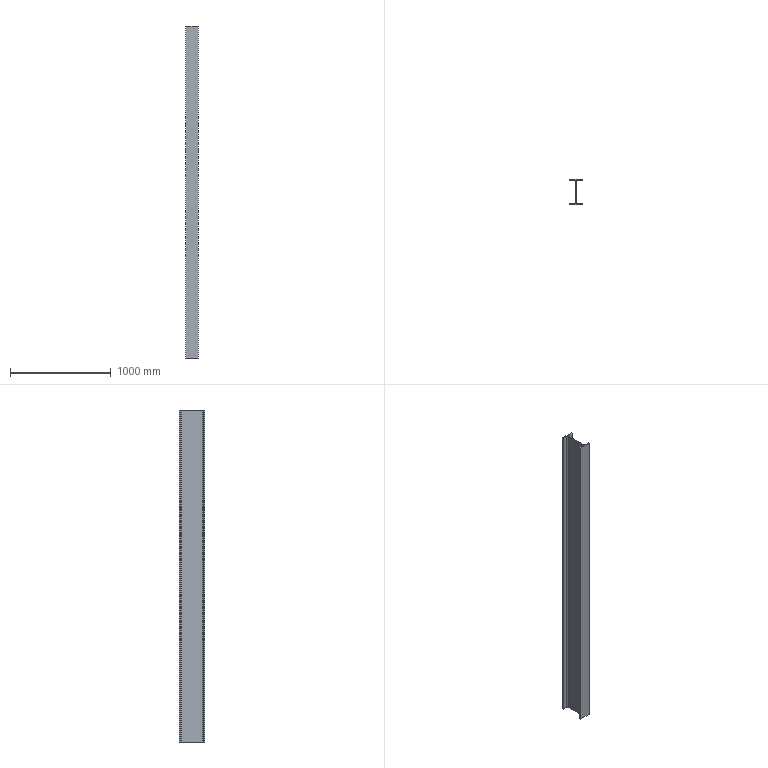Part | SolidWorks | features Extrusion 1 | 1 solid | 18 faces | box 125 x 250 x 3300 mm | volume 12199896 mm3 | plane 14 | cylinder 4 | commonest cylinder face diameters 16 x4
STEP:
#1=CARTESIAN_POINT('',(-62.5,9.,0.));
#2=VERTEX_POINT('',#1);
#3=CARTESIAN_POINT('',(-62.5,0.,0.));
#4=VERTEX_POINT('',#3);
#5=CARTESIAN_POINT('',(-62.5,0.,0.));
#6=DIRECTION('',(0.,-1.,0.));
#7=VECTOR('',#6,1000.);
#8=LINE('',#5,#7);
#9=EDGE_CURVE('',#2,#4,#8,.T.);
#10=ORIENTED_EDGE('',*,*,#9,.T.);
#11=CARTESIAN_POINT('',(-62.5,0.,3300.));
#12=VERTEX_POINT('',#11);
#13=CARTESIAN_POINT('',(-62.5,0.,3300.));
#14=DIRECTION('',(0.,0.,-1.));
#15=VECTOR('',#14,1000.);
#16=LINE('',#13,#15);
#17=EDGE_CURVE('',#12,#4,#16,.T.);
#18=ORIENTED_EDGE('',*,*,#17,.F.);
#19=CARTESIAN_POINT('',(-62.5,9.,3300.));
#20=VERTEX_POINT('',#19);
#21=CARTESIAN_POINT('',(-62.5,0.,3300.));
#22=DIRECTION('',(0.,-1.,0.));
#23=VECTOR('',#22,1000.);
#24=LINE('',#21,#23);
#25=EDGE_CURVE('',#20,#12,#24,.T.);
#26=ORIENTED_EDGE('',*,*,#25,.F.);
#27=CARTESIAN_POINT('',(-62.5,9.,3300.));
#28=DIRECTION('',(0.,0.,-1.));
#29=VECTOR('',#28,1000.);
#30=LINE('',#27,#29);
#31=EDGE_CURVE('',#20,#2,#30,.T.);
#32=ORIENTED_EDGE('',*,*,#31,.T.);
#33=EDGE_LOOP('',(#10,#18,#26,#32));
#34=FACE_OUTER_BOUND('',#33,.T.);
#35=CARTESIAN_POINT('',(-62.5,0.,3300.));
#36=DIRECTION('',(1.,0.,0.));
#37=DIRECTION('',(0.,0.,-1.));
#38=AXIS2_PLACEMENT_3D('',#35,#36,#37);
#39=PLANE('',#38);
#40=ADVANCED_FACE('',(#34),#39,.F.);
#41=CARTESIAN_POINT('',(62.5,0.,0.));
#42=VERTEX_POINT('',#41);
#43=CARTESIAN_POINT('',(62.5,0.,0.));
#44=DIRECTION('',(1.,0.,0.));
#45=VECTOR('',#44,1000.);
#46=LINE('',#43,#45);
#47=EDGE_CURVE('',#4,#42,#46,.T.);
#48=ORIENTED_EDGE('',*,*,#47,.T.);
#49=CARTESIAN_POINT('',(62.5,0.,3300.));
#50=VERTEX_POINT('',#49);
#51=CARTESIAN_POINT('',(62.5,0.,3300.));
#52=DIRECTION('',(0.,0.,-1.));
#53=VECTOR('',#52,1000.);
#54=LINE('',#51,#53);
#55=EDGE_CURVE('',#50,#42,#54,.T.);
#56=ORIENTED_EDGE('',*,*,#55,.F.);
#57=CARTESIAN_POINT('',(62.5,0.,3300.));
#58=DIRECTION('',(1.,0.,0.));
#59=VECTOR('',#58,1000.);
#60=LINE('',#57,#59);
#61=EDGE_CURVE('',#12,#50,#60,.T.);
#62=ORIENTED_EDGE('',*,*,#61,.F.);
#63=ORIENTED_EDGE('',*,*,#17,.T.);
#64=EDGE_LOOP('',(#48,#56,#62,#63));
#65=FACE_OUTER_BOUND('',#64,.T.);
#66=CARTESIAN_POINT('',(62.5,0.,3300.));
#67=DIRECTION('',(0.,1.,0.));
#68=DIRECTION('',(0.,0.,1.));
#69=AXIS2_PLACEMENT_3D('',#66,#67,#68);
#70=PLANE('',#69);
#71=ADVANCED_FACE('',(#65),#70,.F.);
#72=CARTESIAN_POINT('',(62.5,9.,0.));
#73=VERTEX_POINT('',#72);
#74=CARTESIAN_POINT('',(62.5,0.,0.));
#75=DIRECTION('',(0.,1.,0.));
#76=VECTOR('',#75,1000.);
#77=LINE('',#74,#76);
#78=EDGE_CURVE('',#42,#73,#77,.T.);
#79=ORIENTED_EDGE('',*,*,#78,.T.);
#80=CARTESIAN_POINT('',(62.5,9.,3300.));
#81=VERTEX_POINT('',#80);
#82=CARTESIAN_POINT('',(62.5,9.,3300.));
#83=DIRECTION('',(0.,0.,-1.));
#84=VECTOR('',#83,1000.);
#85=LINE('',#82,#84);
#86=EDGE_CURVE('',#81,#73,#85,.T.);
#87=ORIENTED_EDGE('',*,*,#86,.F.);
#88=CARTESIAN_POINT('',(62.5,0.,3300.));
#89=DIRECTION('',(0.,1.,0.));
#90=VECTOR('',#89,1000.);
#91=LINE('',#88,#90);
#92=EDGE_CURVE('',#50,#81,#91,.T.);
#93=ORIENTED_EDGE('',*,*,#92,.F.);
#94=ORIENTED_EDGE('',*,*,#55,.T.);
#95=EDGE_LOOP('',(#79,#87,#93,#94));
#96=FACE_OUTER_BOUND('',#95,.T.);
#97=CARTESIAN_POINT('',(62.5,0.,3300.));
#98=DIRECTION('',(-1.,0.,0.));
#99=DIRECTION('',(0.,0.,1.));
#100=AXIS2_PLACEMENT_3D('',#97,#98,#99);
#101=PLANE('',#100);
#102=ADVANCED_FACE('',(#96),#101,.F.);
#103=CARTESIAN_POINT('',(11.,9.,0.));
#104=VERTEX_POINT('',#103);
#105=CARTESIAN_POINT('',(62.5,9.,0.));
#106=DIRECTION('',(-1.,0.,0.));
#107=VECTOR('',#106,1000.);
#108=LINE('',#105,#107);
#109=EDGE_CURVE('',#73,#104,#108,.T.);
#110=ORIENTED_EDGE('',*,*,#109,.T.);
#111=CARTESIAN_POINT('',(11.,9.,3300.));
#112=VERTEX_POINT('',#111);
#113=CARTESIAN_POINT('',(11.,9.,3300.));
#114=DIRECTION('',(0.,0.,-1.));
#115=VECTOR('',#114,1000.);
#116=LINE('',#113,#115);
#117=EDGE_CURVE('',#112,#104,#116,.T.);
#118=ORIENTED_EDGE('',*,*,#117,.F.);
#119=CARTESIAN_POINT('',(62.5,9.,3300.));
#120=DIRECTION('',(-1.,0.,0.));
#121=VECTOR('',#120,1000.);
#122=LINE('',#119,#121);
#123=EDGE_CURVE('',#81,#112,#122,.T.);
#124=ORIENTED_EDGE('',*,*,#123,.F.);
#125=ORIENTED_EDGE('',*,*,#86,.T.);
#126=EDGE_LOOP('',(#110,#118,#124,#125));
#127=FACE_OUTER_BOUND('',#126,.T.);
#128=CARTESIAN_POINT('',(62.5,9.,3300.));
#129=DIRECTION('',(0.,-1.,0.));
#130=DIRECTION('',(0.,0.,-1.));
#131=AXIS2_PLACEMENT_3D('',#128,#129,#130);
#132=PLANE('',#131);
#133=ADVANCED_FACE('',(#127),#132,.F.);
#134=CARTESIAN_POINT('',(3.,17.,0.));
#135=VERTEX_POINT('',#134);
#136=CARTESIAN_POINT('',(11.,17.,0.));
#137=DIRECTION('',(0.,0.,-1.));
#138=DIRECTION('',(-1.,0.,0.));
#139=AXIS2_PLACEMENT_3D('',#136,#137,#138);
#140=CIRCLE('',#139,8.);
#141=EDGE_CURVE('',#104,#135,#140,.T.);
#142=ORIENTED_EDGE('',*,*,#141,.T.);
#143=CARTESIAN_POINT('',(3.,17.,3300.));
#144=VERTEX_POINT('',#143);
#145=CARTESIAN_POINT('',(3.,17.,3300.));
#146=DIRECTION('',(0.,0.,-1.));
#147=VECTOR('',#146,1000.);
#148=LINE('',#145,#147);
#149=EDGE_CURVE('',#144,#135,#148,.T.);
#150=ORIENTED_EDGE('',*,*,#149,.F.);
#151=CARTESIAN_POINT('',(11.,17.,3300.));
#152=DIRECTION('',(0.,0.,-1.));
#153=DIRECTION('',(-1.,0.,0.));
#154=AXIS2_PLACEMENT_3D('',#151,#152,#153);
#155=CIRCLE('',#154,8.);
#156=EDGE_CURVE('',#112,#144,#155,.T.);
#157=ORIENTED_EDGE('',*,*,#156,.F.);
#158=ORIENTED_EDGE('',*,*,#117,.T.);
#159=EDGE_LOOP('',(#142,#150,#157,#158));
#160=FACE_OUTER_BOUND('',#159,.T.);
#161=CARTESIAN_POINT('',(11.,17.,3300.));
#162=DIRECTION('',(0.,0.,-1.));
#163=DIRECTION('',(-1.,0.,0.));
#164=AXIS2_PLACEMENT_3D('',#161,#162,#163);
#165=CYLINDRICAL_SURFACE('',#164,8.);
#166=ADVANCED_FACE('',(#160),#165,.F.);
#167=CARTESIAN_POINT('',(3.,233.,0.));
#168=VERTEX_POINT('',#167);
#169=CARTESIAN_POINT('',(3.,17.,0.));
#170=DIRECTION('',(0.,1.,0.));
#171=VECTOR('',#170,1000.);
#172=LINE('',#169,#171);
#173=EDGE_CURVE('',#135,#168,#172,.T.);
#174=ORIENTED_EDGE('',*,*,#173,.T.);
#175=CARTESIAN_POINT('',(3.,233.,3300.));
#176=VERTEX_POINT('',#175);
#177=CARTESIAN_POINT('',(3.,233.,3300.));
#178=DIRECTION('',(0.,0.,-1.));
#179=VECTOR('',#178,1000.);
#180=LINE('',#177,#179);
#181=EDGE_CURVE('',#176,#168,#180,.T.);
#182=ORIENTED_EDGE('',*,*,#181,.F.);
#183=CARTESIAN_POINT('',(3.,17.,3300.));
#184=DIRECTION('',(0.,1.,0.));
#185=VECTOR('',#184,1000.);
#186=LINE('',#183,#185);
#187=EDGE_CURVE('',#144,#176,#186,.T.);
#188=ORIENTED_EDGE('',*,*,#187,.F.);
#189=ORIENTED_EDGE('',*,*,#149,.T.);
#190=EDGE_LOOP('',(#174,#182,#188,#189));
#191=FACE_OUTER_BOUND('',#190,.T.);
#192=CARTESIAN_POINT('',(3.,17.,3300.));
#193=DIRECTION('',(-1.,0.,0.));
#194=DIRECTION('',(0.,-1.,0.));
#195=AXIS2_PLACEMENT_3D('',#192,#193,#194);
#196=PLANE('',#195);
#197=ADVANCED_FACE('',(#191),#196,.F.);
#198=CARTESIAN_POINT('',(11.,241.,0.));
#199=VERTEX_POINT('',#198);
#200=CARTESIAN_POINT('',(11.,233.,0.));
#201=DIRECTION('',(0.,0.,-1.));
#202=DIRECTION('',(-1.,0.,0.));
#203=AXIS2_PLACEMENT_3D('',#200,#201,#202);
#204=CIRCLE('',#203,8.);
#205=EDGE_CURVE('',#168,#199,#204,.T.);
#206=ORIENTED_EDGE('',*,*,#205,.T.);
#207=CARTESIAN_POINT('',(11.,241.,3300.));
#208=VERTEX_POINT('',#207);
#209=CARTESIAN_POINT('',(11.,241.,3300.));
#210=DIRECTION('',(0.,0.,-1.));
#211=VECTOR('',#210,1000.);
#212=LINE('',#209,#211);
#213=EDGE_CURVE('',#208,#199,#212,.T.);
#214=ORIENTED_EDGE('',*,*,#213,.F.);
#215=CARTESIAN_POINT('',(11.,233.,3300.));
#216=DIRECTION('',(0.,0.,-1.));
#217=DIRECTION('',(-1.,0.,0.));
#218=AXIS2_PLACEMENT_3D('',#215,#216,#217);
#219=CIRCLE('',#218,8.);
#220=EDGE_CURVE('',#176,#208,#219,.T.);
#221=ORIENTED_EDGE('',*,*,#220,.F.);
#222=ORIENTED_EDGE('',*,*,#181,.T.);
#223=EDGE_LOOP('',(#206,#214,#221,#222));
#224=FACE_OUTER_BOUND('',#223,.T.);
#225=CARTESIAN_POINT('',(11.,233.,3300.));
#226=DIRECTION('',(0.,0.,-1.));
#227=DIRECTION('',(-1.,0.,0.));
#228=AXIS2_PLACEMENT_3D('',#225,#226,#227);
#229=CYLINDRICAL_SURFACE('',#228,8.);
#230=ADVANCED_FACE('',(#224),#229,.F.);
#231=CARTESIAN_POINT('',(62.5,241.,0.));
#232=VERTEX_POINT('',#231);
#233=CARTESIAN_POINT('',(11.,241.,0.));
#234=DIRECTION('',(1.,0.,0.));
#235=VECTOR('',#234,1000.);
#236=LINE('',#233,#235);
#237=EDGE_CURVE('',#199,#232,#236,.T.);
#238=ORIENTED_EDGE('',*,*,#237,.T.);
#239=CARTESIAN_POINT('',(62.5,241.,3300.));
#240=VERTEX_POINT('',#239);
#241=CARTESIAN_POINT('',(62.5,241.,3300.));
#242=DIRECTION('',(0.,0.,-1.));
#243=VECTOR('',#242,1000.);
#244=LINE('',#241,#243);
#245=EDGE_CURVE('',#240,#232,#244,.T.);
#246=ORIENTED_EDGE('',*,*,#245,.F.);
#247=CARTESIAN_POINT('',(11.,241.,3300.));
#248=DIRECTION('',(1.,0.,0.));
#249=VECTOR('',#248,1000.);
#250=LINE('',#247,#249);
#251=EDGE_CURVE('',#208,#240,#250,.T.);
#252=ORIENTED_EDGE('',*,*,#251,.F.);
#253=ORIENTED_EDGE('',*,*,#213,.T.);
#254=EDGE_LOOP('',(#238,#246,#252,#253));
#255=FACE_OUTER_BOUND('',#254,.T.);
#256=CARTESIAN_POINT('',(11.,241.,3300.));
#257=DIRECTION('',(0.,1.,0.));
#258=DIRECTION('',(0.,0.,1.));
#259=AXIS2_PLACEMENT_3D('',#256,#257,#258);
#260=PLANE('',#259);
#261=ADVANCED_FACE('',(#255),#260,.F.);
#262=CARTESIAN_POINT('',(62.5,250.,0.));
#263=VERTEX_POINT('',#262);
#264=CARTESIAN_POINT('',(62.5,241.,0.));
#265=DIRECTION('',(0.,1.,0.));
#266=VECTOR('',#265,1000.);
#267=LINE('',#264,#266);
#268=EDGE_CURVE('',#232,#263,#267,.T.);
#269=ORIENTED_EDGE('',*,*,#268,.T.);
#270=CARTESIAN_POINT('',(62.5,250.,3300.));
#271=VERTEX_POINT('',#270);
#272=CARTESIAN_POINT('',(62.5,250.,3300.));
#273=DIRECTION('',(0.,0.,-1.));
#274=VECTOR('',#273,1000.);
#275=LINE('',#272,#274);
#276=EDGE_CURVE('',#271,#263,#275,.T.);
#277=ORIENTED_EDGE('',*,*,#276,.F.);
#278=CARTESIAN_POINT('',(62.5,241.,3300.));
#279=DIRECTION('',(0.,1.,0.));
#280=VECTOR('',#279,1000.);
#281=LINE('',#278,#280);
#282=EDGE_CURVE('',#240,#271,#281,.T.);
#283=ORIENTED_EDGE('',*,*,#282,.F.);
#284=ORIENTED_EDGE('',*,*,#245,.T.);
#285=EDGE_LOOP('',(#269,#277,#283,#284));
#286=FACE_OUTER_BOUND('',#285,.T.);
#287=CARTESIAN_POINT('',(62.5,241.,3300.));
#288=DIRECTION('',(-1.,0.,0.));
#289=DIRECTION('',(0.,0.,1.));
#290=AXIS2_PLACEMENT_3D('',#287,#288,#289);
#291=PLANE('',#290);
#292=ADVANCED_FACE('',(#286),#291,.F.);
#293=CARTESIAN_POINT('',(-62.5,250.,0.));
#294=VERTEX_POINT('',#293);
#295=CARTESIAN_POINT('',(-62.5,250.,0.));
#296=DIRECTION('',(-1.,0.,0.));
#297=VECTOR('',#296,1000.);
#298=LINE('',#295,#297);
#299=EDGE_CURVE('',#263,#294,#298,.T.);
#300=ORIENTED_EDGE('',*,*,#299,.T.);
#301=CARTESIAN_POINT('',(-62.5,250.,3300.));
#302=VERTEX_POINT('',#301);
#303=CARTESIAN_POINT('',(-62.5,250.,3300.));
#304=DIRECTION('',(0.,0.,-1.));
#305=VECTOR('',#304,1000.);
#306=LINE('',#303,#305);
#307=EDGE_CURVE('',#302,#294,#306,.T.);
#308=ORIENTED_EDGE('',*,*,#307,.F.);
#309=CARTESIAN_POINT('',(-62.5,250.,3300.));
#310=DIRECTION('',(-1.,0.,0.));
#311=VECTOR('',#310,1000.);
#312=LINE('',#309,#311);
#313=EDGE_CURVE('',#271,#302,#312,.T.);
#314=ORIENTED_EDGE('',*,*,#313,.F.);
#315=ORIENTED_EDGE('',*,*,#276,.T.);
#316=EDGE_LOOP('',(#300,#308,#314,#315));
#317=FACE_OUTER_BOUND('',#316,.T.);
#318=CARTESIAN_POINT('',(-62.5,250.,3300.));
#319=DIRECTION('',(0.,-1.,0.));
#320=DIRECTION('',(1.,0.,0.));
#321=AXIS2_PLACEMENT_3D('',#318,#319,#320);
#322=PLANE('',#321);
#323=ADVANCED_FACE('',(#317),#322,.F.);
#324=CARTESIAN_POINT('',(-62.5,241.,0.));
#325=VERTEX_POINT('',#324);
#326=CARTESIAN_POINT('',(-62.5,241.,0.));
#327=DIRECTION('',(0.,-1.,0.));
#328=VECTOR('',#327,1000.);
#329=LINE('',#326,#328);
#330=EDGE_CURVE('',#294,#325,#329,.T.);
#331=ORIENTED_EDGE('',*,*,#330,.T.);
#332=CARTESIAN_POINT('',(-62.5,241.,3300.));
#333=VERTEX_POINT('',#332);
#334=CARTESIAN_POINT('',(-62.5,241.,3300.));
#335=DIRECTION('',(0.,0.,-1.));
#336=VECTOR('',#335,1000.);
#337=LINE('',#334,#336);
#338=EDGE_CURVE('',#333,#325,#337,.T.);
#339=ORIENTED_EDGE('',*,*,#338,.F.);
#340=CARTESIAN_POINT('',(-62.5,241.,3300.));
#341=DIRECTION('',(0.,-1.,0.));
#342=VECTOR('',#341,1000.);
#343=LINE('',#340,#342);
#344=EDGE_CURVE('',#302,#333,#343,.T.);
#345=ORIENTED_EDGE('',*,*,#344,.F.);
#346=ORIENTED_EDGE('',*,*,#307,.T.);
#347=EDGE_LOOP('',(#331,#339,#345,#346));
#348=FACE_OUTER_BOUND('',#347,.T.);
#349=CARTESIAN_POINT('',(-62.5,241.,3300.));
#350=DIRECTION('',(1.,0.,0.));
#351=DIRECTION('',(0.,0.,-1.));
#352=AXIS2_PLACEMENT_3D('',#349,#350,#351);
#353=PLANE('',#352);
#354=ADVANCED_FACE('',(#348),#353,.F.);
#355=CARTESIAN_POINT('',(-11.,241.,0.));
#356=VERTEX_POINT('',#355);
#357=CARTESIAN_POINT('',(-11.,241.,0.));
#358=DIRECTION('',(1.,0.,0.));
#359=VECTOR('',#358,1000.);
#360=LINE('',#357,#359);
#361=EDGE_CURVE('',#325,#356,#360,.T.);
#362=ORIENTED_EDGE('',*,*,#361,.T.);
#363=CARTESIAN_POINT('',(-11.,241.,3300.));
#364=VERTEX_POINT('',#363);
#365=CARTESIAN_POINT('',(-11.,241.,3300.));
#366=DIRECTION('',(0.,0.,-1.));
#367=VECTOR('',#366,1000.);
#368=LINE('',#365,#367);
#369=EDGE_CURVE('',#364,#356,#368,.T.);
#370=ORIENTED_EDGE('',*,*,#369,.F.);
#371=CARTESIAN_POINT('',(-11.,241.,3300.));
#372=DIRECTION('',(1.,0.,0.));
#373=VECTOR('',#372,1000.);
#374=LINE('',#371,#373);
#375=EDGE_CURVE('',#333,#364,#374,.T.);
#376=ORIENTED_EDGE('',*,*,#375,.F.);
#377=ORIENTED_EDGE('',*,*,#338,.T.);
#378=EDGE_LOOP('',(#362,#370,#376,#377));
#379=FACE_OUTER_BOUND('',#378,.T.);
#380=CARTESIAN_POINT('',(-11.,241.,3300.));
#381=DIRECTION('',(0.,1.,0.));
#382=DIRECTION('',(0.,0.,1.));
#383=AXIS2_PLACEMENT_3D('',#380,#381,#382);
#384=PLANE('',#383);
#385=ADVANCED_FACE('',(#379),#384,.F.);
#386=CARTESIAN_POINT('',(-3.,233.,0.));
#387=VERTEX_POINT('',#386);
#388=CARTESIAN_POINT('',(-11.,233.,0.));
#389=DIRECTION('',(0.,0.,-1.));
#390=DIRECTION('',(1.,0.,0.));
#391=AXIS2_PLACEMENT_3D('',#388,#389,#390);
#392=CIRCLE('',#391,8.);
#393=EDGE_CURVE('',#356,#387,#392,.T.);
#394=ORIENTED_EDGE('',*,*,#393,.T.);
#395=CARTESIAN_POINT('',(-3.,233.,3300.));
#396=VERTEX_POINT('',#395);
#397=CARTESIAN_POINT('',(-3.,233.,3300.));
#398=DIRECTION('',(0.,0.,-1.));
#399=VECTOR('',#398,1000.);
#400=LINE('',#397,#399);
#401=EDGE_CURVE('',#396,#387,#400,.T.);
#402=ORIENTED_EDGE('',*,*,#401,.F.);
#403=CARTESIAN_POINT('',(-11.,233.,3300.));
#404=DIRECTION('',(0.,0.,-1.));
#405=DIRECTION('',(1.,0.,0.));
#406=AXIS2_PLACEMENT_3D('',#403,#404,#405);
#407=CIRCLE('',#406,8.);
#408=EDGE_CURVE('',#364,#396,#407,.T.);
#409=ORIENTED_EDGE('',*,*,#408,.F.);
#410=ORIENTED_EDGE('',*,*,#369,.T.);
#411=EDGE_LOOP('',(#394,#402,#409,#410));
#412=FACE_OUTER_BOUND('',#411,.T.);
#413=CARTESIAN_POINT('',(-11.,233.,3300.));
#414=DIRECTION('',(0.,0.,-1.));
#415=DIRECTION('',(-1.,0.,0.));
#416=AXIS2_PLACEMENT_3D('',#413,#414,#415);
#417=CYLINDRICAL_SURFACE('',#416,8.);
#418=ADVANCED_FACE('',(#412),#417,.F.);
#419=CARTESIAN_POINT('',(-3.,17.,0.));
#420=VERTEX_POINT('',#419);
#421=CARTESIAN_POINT('',(-3.,17.,0.));
#422=DIRECTION('',(0.,-1.,0.));
#423=VECTOR('',#422,1000.);
#424=LINE('',#421,#423);
#425=EDGE_CURVE('',#387,#420,#424,.T.);
#426=ORIENTED_EDGE('',*,*,#425,.T.);
#427=CARTESIAN_POINT('',(-3.,17.,3300.));
#428=VERTEX_POINT('',#427);
#429=CARTESIAN_POINT('',(-3.,17.,3300.));
#430=DIRECTION('',(0.,0.,-1.));
#431=VECTOR('',#430,1000.);
#432=LINE('',#429,#431);
#433=EDGE_CURVE('',#428,#420,#432,.T.);
#434=ORIENTED_EDGE('',*,*,#433,.F.);
#435=CARTESIAN_POINT('',(-3.,17.,3300.));
#436=DIRECTION('',(0.,-1.,0.));
#437=VECTOR('',#436,1000.);
#438=LINE('',#435,#437);
#439=EDGE_CURVE('',#396,#428,#438,.T.);
#440=ORIENTED_EDGE('',*,*,#439,.F.);
#441=ORIENTED_EDGE('',*,*,#401,.T.);
#442=EDGE_LOOP('',(#426,#434,#440,#441));
#443=FACE_OUTER_BOUND('',#442,.T.);
#444=CARTESIAN_POINT('',(-3.,17.,3300.));
#445=DIRECTION('',(1.,0.,0.));
#446=DIRECTION('',(0.,1.,0.));
#447=AXIS2_PLACEMENT_3D('',#444,#445,#446);
#448=PLANE('',#447);
#449=ADVANCED_FACE('',(#443),#448,.F.);
#450=CARTESIAN_POINT('',(-11.,9.,0.));
#451=VERTEX_POINT('',#450);
#452=CARTESIAN_POINT('',(-11.,17.,0.));
#453=DIRECTION('',(0.,0.,-1.));
#454=DIRECTION('',(-1.,0.,0.));
#455=AXIS2_PLACEMENT_3D('',#452,#453,#454);
#456=CIRCLE('',#455,8.);
#457=EDGE_CURVE('',#420,#451,#456,.T.);
#458=ORIENTED_EDGE('',*,*,#457,.T.);
#459=CARTESIAN_POINT('',(-11.,9.,3300.));
#460=VERTEX_POINT('',#459);
#461=CARTESIAN_POINT('',(-11.,9.,3300.));
#462=DIRECTION('',(0.,0.,-1.));
#463=VECTOR('',#462,1000.);
#464=LINE('',#461,#463);
#465=EDGE_CURVE('',#460,#451,#464,.T.);
#466=ORIENTED_EDGE('',*,*,#465,.F.);
#467=CARTESIAN_POINT('',(-11.,17.,3300.));
#468=DIRECTION('',(0.,0.,-1.));
#469=DIRECTION('',(-1.,0.,0.));
#470=AXIS2_PLACEMENT_3D('',#467,#468,#469);
#471=CIRCLE('',#470,8.);
#472=EDGE_CURVE('',#428,#460,#471,.T.);
#473=ORIENTED_EDGE('',*,*,#472,.F.);
#474=ORIENTED_EDGE('',*,*,#433,.T.);
#475=EDGE_LOOP('',(#458,#466,#473,#474));
#476=FACE_OUTER_BOUND('',#475,.T.);
#477=CARTESIAN_POINT('',(-11.,17.,3300.));
#478=DIRECTION('',(0.,0.,-1.));
#479=DIRECTION('',(-1.,0.,0.));
#480=AXIS2_PLACEMENT_3D('',#477,#478,#479);
#481=CYLINDRICAL_SURFACE('',#480,8.);
#482=ADVANCED_FACE('',(#476),#481,.F.);
#483=CARTESIAN_POINT('',(-62.5,9.,0.));
#484=DIRECTION('',(-1.,0.,0.));
#485=VECTOR('',#484,1000.);
#486=LINE('',#483,#485);
#487=EDGE_CURVE('',#451,#2,#486,.T.);
#488=ORIENTED_EDGE('',*,*,#487,.T.);
#489=ORIENTED_EDGE('',*,*,#31,.F.);
#490=CARTESIAN_POINT('',(-62.5,9.,3300.));
#491=DIRECTION('',(-1.,0.,0.));
#492=VECTOR('',#491,1000.);
#493=LINE('',#490,#492);
#494=EDGE_CURVE('',#460,#20,#493,.T.);
#495=ORIENTED_EDGE('',*,*,#494,.F.);
#496=ORIENTED_EDGE('',*,*,#465,.T.);
#497=EDGE_LOOP('',(#488,#489,#495,#496));
#498=FACE_OUTER_BOUND('',#497,.T.);
#499=CARTESIAN_POINT('',(-62.5,9.,3300.));
#500=DIRECTION('',(0.,-1.,0.));
#501=DIRECTION('',(0.,0.,-1.));
#502=AXIS2_PLACEMENT_3D('',#499,#500,#501);
#503=PLANE('',#502);
#504=ADVANCED_FACE('',(#498),#503,.F.);
#505=ORIENTED_EDGE('',*,*,#25,.T.);
#506=ORIENTED_EDGE('',*,*,#61,.T.);
#507=ORIENTED_EDGE('',*,*,#92,.T.);
#508=ORIENTED_EDGE('',*,*,#123,.T.);
#509=ORIENTED_EDGE('',*,*,#156,.T.);
#510=ORIENTED_EDGE('',*,*,#187,.T.);
#511=ORIENTED_EDGE('',*,*,#220,.T.);
#512=ORIENTED_EDGE('',*,*,#251,.T.);
#513=ORIENTED_EDGE('',*,*,#282,.T.);
#514=ORIENTED_EDGE('',*,*,#313,.T.);
#515=ORIENTED_EDGE('',*,*,#344,.T.);
#516=ORIENTED_EDGE('',*,*,#375,.T.);
#517=ORIENTED_EDGE('',*,*,#408,.T.);
#518=ORIENTED_EDGE('',*,*,#439,.T.);
#519=ORIENTED_EDGE('',*,*,#472,.T.);
#520=ORIENTED_EDGE('',*,*,#494,.T.);
#521=EDGE_LOOP('',(#505,#506,#507,#508,#509,#510,#511,#512,#513,#514,#515,#516,#517,#518,#519,#520));
#522=FACE_OUTER_BOUND('',#521,.T.);
#523=CARTESIAN_POINT('',(-11.,17.,3300.));
#524=DIRECTION('',(0.,0.,-1.));
#525=DIRECTION('',(-1.,0.,0.));
#526=AXIS2_PLACEMENT_3D('',#523,#524,#525);
#527=PLANE('',#526);
#528=ADVANCED_FACE('',(#522),#527,.F.);
#529=ORIENTED_EDGE('',*,*,#9,.F.);
#530=ORIENTED_EDGE('',*,*,#487,.F.);
#531=ORIENTED_EDGE('',*,*,#457,.F.);
#532=ORIENTED_EDGE('',*,*,#425,.F.);
#533=ORIENTED_EDGE('',*,*,#393,.F.);
#534=ORIENTED_EDGE('',*,*,#361,.F.);
#535=ORIENTED_EDGE('',*,*,#330,.F.);
#536=ORIENTED_EDGE('',*,*,#299,.F.);
#537=ORIENTED_EDGE('',*,*,#268,.F.);
#538=ORIENTED_EDGE('',*,*,#237,.F.);
#539=ORIENTED_EDGE('',*,*,#205,.F.);
#540=ORIENTED_EDGE('',*,*,#173,.F.);
#541=ORIENTED_EDGE('',*,*,#141,.F.);
#542=ORIENTED_EDGE('',*,*,#109,.F.);
#543=ORIENTED_EDGE('',*,*,#78,.F.);
#544=ORIENTED_EDGE('',*,*,#47,.F.);
#545=EDGE_LOOP('',(#529,#530,#531,#532,#533,#534,#535,#536,#537,#538,#539,#540,#541,#542,#543,#544));
#546=FACE_OUTER_BOUND('',#545,.T.);
#547=CARTESIAN_POINT('',(-11.,17.,0.));
#548=DIRECTION('',(0.,0.,-1.));
#549=DIRECTION('',(-1.,0.,0.));
#550=AXIS2_PLACEMENT_3D('',#547,#548,#549);
#551=PLANE('',#550);
#552=ADVANCED_FACE('',(#546),#551,.T.);
#553=CLOSED_SHELL('',(#40,#71,#102,#133,#166,#197,#230,#261,#292,#323,#354,#385,#418,#449,#482,#504,#528,#552));
#554=MANIFOLD_SOLID_BREP('',#553);
#555=CARTESIAN_POINT('',(0.,0.,0.));
#556=DIRECTION('',(0.,0.,1.));
#557=DIRECTION('',(1.,0.,0.));
#558=AXIS2_PLACEMENT_3D('',#555,#556,#557);
#559=(LENGTH_UNIT()NAMED_UNIT(*)SI_UNIT(.MILLI.,.METRE.));
#560=UNCERTAINTY_MEASURE_WITH_UNIT(LENGTH_MEASURE(0.00001),#559,'','');
#561=(NAMED_UNIT(*)PLANE_ANGLE_UNIT()SI_UNIT($,.RADIAN.));
#562=(NAMED_UNIT(*)SI_UNIT($,.STERADIAN.)SOLID_ANGLE_UNIT());
#563=(GEOMETRIC_REPRESENTATION_CONTEXT(3)GLOBAL_UNCERTAINTY_ASSIGNED_CONTEXT((#560))GLOBAL_UNIT_ASSIGNED_CONTEXT((#559,#561,#562))REPRESENTATION_CONTEXT('',''));
#564=ADVANCED_BREP_SHAPE_REPRESENTATION('',(#554,#558),#563);